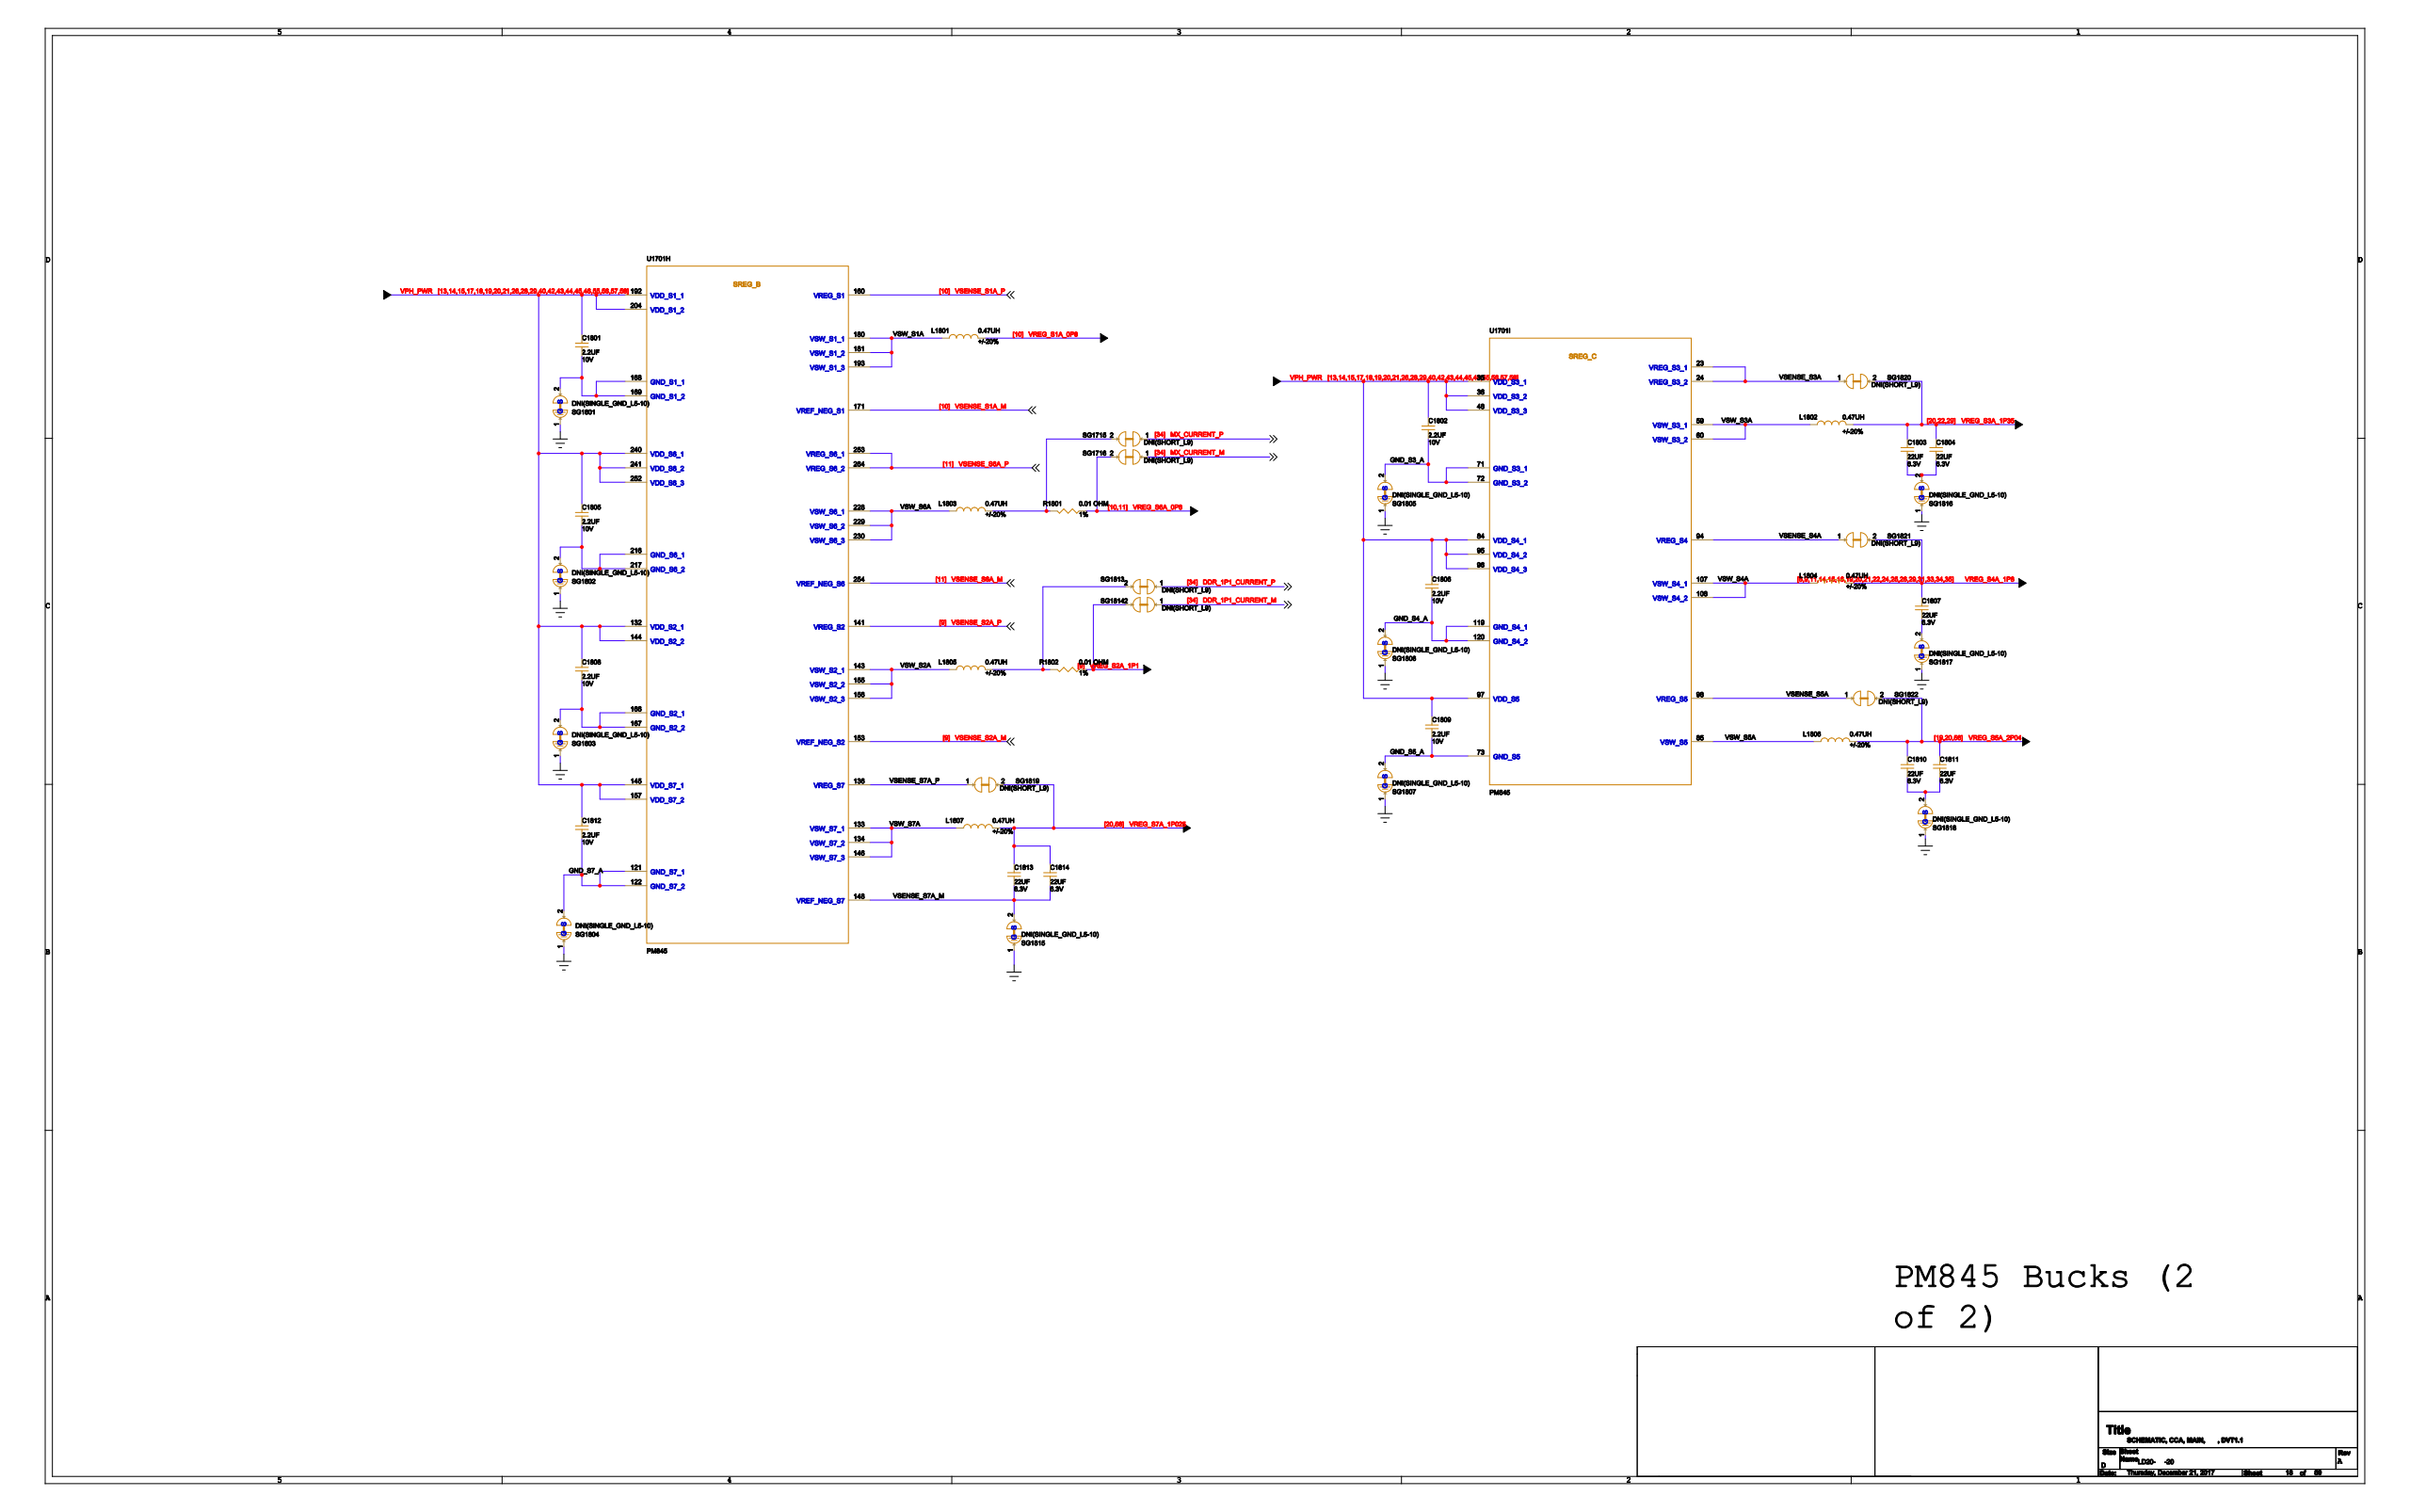Circuit board | Cadence Allegro | 1520 parts | 1149 nets | one sheet of the schematic
Parts on this sheet (reference | value | footprint):
C1801 | 2.2UF | 2P0201R
C1802 | 2.2UF | 2P0201R
C1803 | 22UF | 2P0603R
C1804 | 22UF | 2P0603R
C1805 | 2.2UF | 2P0201R
C1806 | 2.2UF | 2P0201R
C1807 | 22UF | 2P0603R
C1808 | 2.2UF | 2P0201R
C1809 | 2.2UF | 2P0201R
C1810 | 22UF | 2P0603R
C1811 | 22UF | 2P0603R
C1812 | 2.2UF | 2P0201R
C1813 | 22UF | 2P0603R
C1814 | 22UF | 2P0603R
L1801 | 0.47UH | 2PSM87X71NV2
L1802 | 0.47UH | 2PSM87X71NV2
L1803 | 0.47UH | 2PSM87X71NV2
L1804 | 0.47UH | 2PSM87X71NV2
L1805 | 0.47UH | 2PSM87X71NV2
L1806 | 0.47UH | 2PSM87X71NV2
L1807 | 0.47UH | 2PSM87X71NV2
R1801 | 0.01 OHM | 2P0603R
R1802 | 0.01 OHM | 2P0603R
SG1715 | DNI(SHORT_L9) | SHORT_L9_2REC08X12
SG1716 | DNI(SHORT_L9) | SHORT_L9_2REC08X12
SG1801 | DNI(SINGLE_GND_L5-10) | GND_L5-10
SG1802 | DNI(SINGLE_GND_L5-10) | GND_L5-10
SG1803 | DNI(SINGLE_GND_L5-10) | GND_L5-10
SG1804 | DNI(SINGLE_GND_L5-10) | GND_L5-10
SG1805 | DNI(SINGLE_GND_L5-10) | GND_L5-10
SG1806 | DNI(SINGLE_GND_L5-10) | GND_L5-10
SG1807 | DNI(SINGLE_GND_L5-10) | GND_L5-10
SG1813 | DNI(SHORT_L9) | SHORT_L9_2REC08X12
SG1814 | DNI(SHORT_L9) | SHORT_L9_2REC08X12
SG1815 | DNI(SINGLE_GND_L5-10) | GND_L5-10
SG1816 | DNI(SINGLE_GND_L5-10) | GND_L5-10
SG1817 | DNI(SINGLE_GND_L5-10) | GND_L5-10
SG1818 | DNI(SINGLE_GND_L5-10) | GND_L5-10
SG1819 | DNI(SHORT_L9) | SHORT_L9_2REC08X12
SG1820 | DNI(SHORT_L9) | SHORT_L9_2REC08X12
SG1821 | DNI(SHORT_L9) | SHORT_L9_2REC08X12
SG1822 | DNI(SHORT_L9) | SHORT_L9_2REC08X12
U1701 | PM845 | 287PGA242X240B138D45
Nets of these parts (net: part-pin ...):
GND: SG1801-1 SG1802-1 SG1803-1 SG1804-1 SG1805-1 SG1806-1 SG1807-1 SG1815-1 SG1816-1 SG1817-1 SG1818-1
VREG_S4A_1P8: C1807-1 L1804-2 SG1821-2 U1701-57
N34060555: C1801-2 SG1801-2 U1701-168 U1701-169
N34060645: C1805-2 SG1802-2 U1701-216 U1701-217
N34060675: C1808-2 SG1803-2 U1701-166 U1701-167
GND_S7_A: C1812-2 SG1804-2 U1701-121 U1701-122
GND_S3_A: C1802-2 SG1805-2 U1701-71 U1701-72
GND_S4_A: C1806-2 SG1806-2 U1701-119 U1701-120
GND_S5_A: C1809-2 SG1807-2 U1701-73
VSENSE_S7A_M: C1813-2 C1814-2 SG1815-2 U1701-148
N34063267: C1803-2 C1804-2 SG1816-2
N34063462: C1807-2 SG1817-2
N34063540: C1810-2 C1811-2 SG1818-2
VREG_S7A_1P025: C1813-1 C1814-1 L1807-2 SG1819-2
VREG_S5A_2P04: C1810-1 C1811-1 L1806-2 SG1822-2 U1701-29
VPH_PWR: C1801-1 C1802-1 C1805-1 C1806-1 C1808-1 C1809-1 C1812-1 U1701-35 U1701-36 U1701-48 U1701-56 U1701-84 U1701-95 U1701-96 U1701-97 U1701-132 U1701-144 U1701-145 U1701-157 U1701-192 U1701-204 U1701-240 U1701-241 U1701-252
VREG_S3A_1P35: C1803-1 C1804-1 L1802-2 SG1820-2 U1701-22 U1701-33
VSENSE_S7A_P: SG1819-1 U1701-136
VSENSE_S3A: SG1820-1 U1701-23 U1701-24
VSENSE_S4A: SG1821-1 U1701-94
VSENSE_S5A: SG1822-1 U1701-98
MX_CURRENT_P: SG1715-1
N47080619: L1803-2 R1801-1 SG1715-2
MX_CURRENT_M: SG1716-1
VREG_S6A_0P8: R1801-2 SG1716-2
DDR_1P1_CURRENT_P: SG1813-1
N34910709: L1805-2 R1802-1 SG1813-2
DDR_1P1_CURRENT_M: SG1814-1
VREG_S2A_1P1: R1802-2 SG1814-2
VREG_S1A_0P8: L1801-2
VSENSE_S2A_M: U1701-153
VSENSE_S2A_P: U1701-141
VSENSE_S1A_M: U1701-171
VSENSE_S1A_P: U1701-160
VSENSE_S6A_M: U1701-254
VSENSE_S6A_P: U1701-253 U1701-264
VSW_S3A: L1802-1 U1701-59 U1701-60
VSW_S5A: L1806-1 U1701-85
VSW_S1A: L1801-1 U1701-180 U1701-181 U1701-193
VSW_S6A: L1803-1 U1701-228 U1701-229 U1701-230
VSW_S4A: L1804-1 U1701-107 U1701-108
VSW_S2A: L1805-1 U1701-143 U1701-155 U1701-156
VSW_S7A: L1807-1 U1701-133 U1701-134 U1701-146